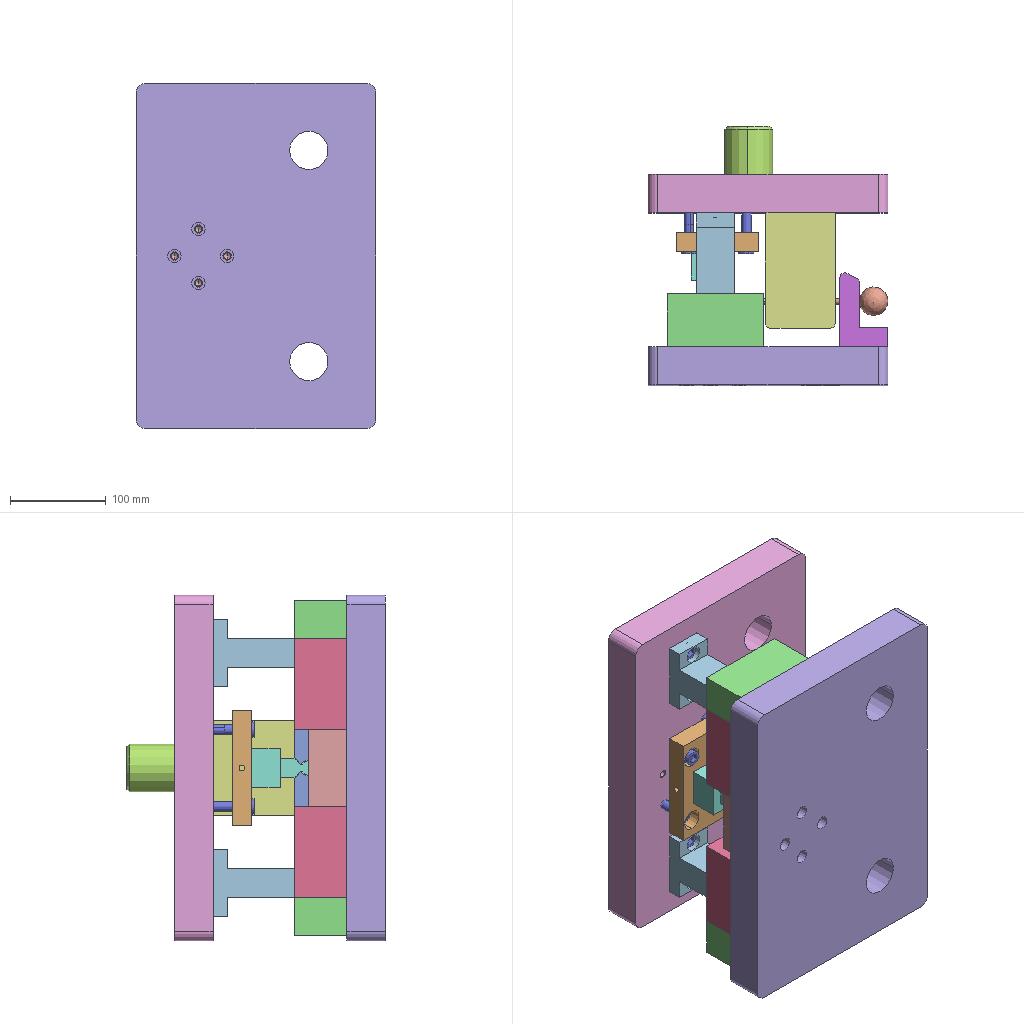Assembly | SolidWorks | 15 different items | 46 placed | box 250 x 270 x 360 mm
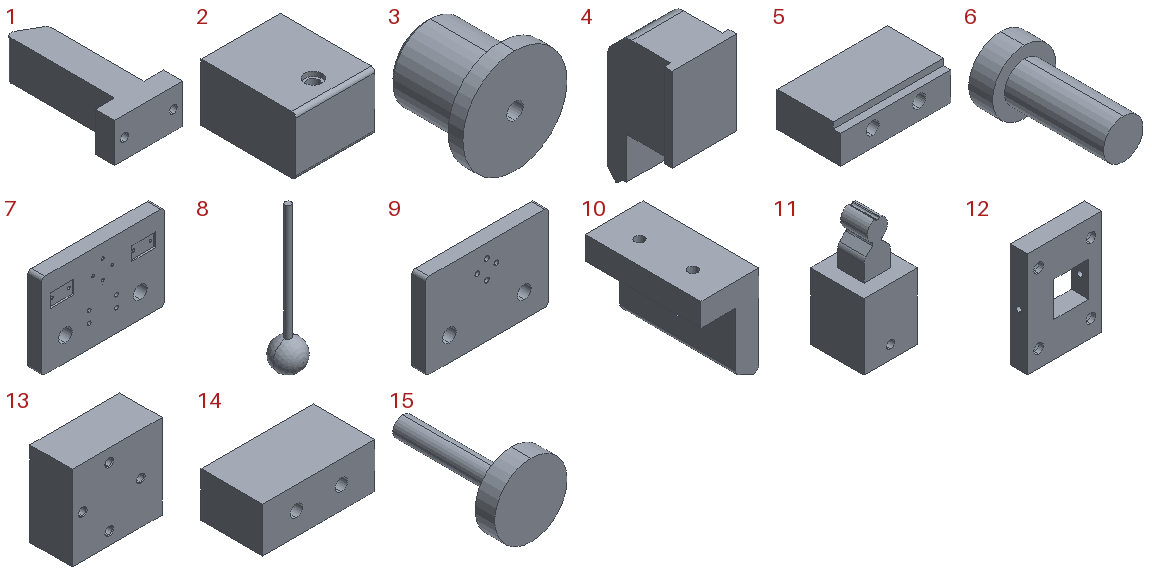Parts list (item | quantity | size | volume | features):
1 | x2 | 70 x 131.42 x 40 mm | 176977 mm3 | features ICE 3, Extrusion 1, Fillet 1, MoveFace 1
2 | x1 | 100 x 120 x 73 mm | 861044 mm3 | features ICE 3, MoveFace 2, Extrusion 1, Fillet 1, HoleWzd 1
3 | x1 | 70 x 60 x 70 mm | 128525 mm3 | features ICE 3, Chamfer 1, Extrusion 1
4 | x2 | 50 x 55 x 101.25 mm | 146000 mm3 | features ICE 3, Extrusion 1, Fillet 1
5 | x4 | 95 x 55 x 30 mm | 136523 mm3 | features ICE 3, Extrusion 1
6 | x26 | 16 x 31 x 16 mm | 2781 mm3 | features ICE 2, Extrusion 1
7 | x1 | 360 x 40 x 250 mm | 3399015 mm3 | features ICE 4, HoleWzd 3, Extrusion 1, MoveFace 1
8 | x1 | 30 x 30 x 145 mm | 17393 mm3 | features ICE 1, Revolution 1
9 | x1 | 360 x 40 x 250 mm | 3459963 mm3 | features Extrusion 1, HoleWzd 1, ICE 1
10 | x1 | 50 x 100 x 76.91 mm | 202541 mm3 | features ICE 4, Extrusion 1, Fillet 1
11 | x1 | 40 x 40 x 87.456 mm | 90363 mm3 | features ICE 3, Extrusion 1
12 | x1 | 85 x 20 x 120 mm | 147044 mm3 | features ICE 2, Extrusion 1
13 | x1 | 85 x 40 x 80 mm | 265399 mm3 | features ICE 2, Extrusion 1, HoleWzd 1
14 | x2 | 100 x 55 x 40 mm | 203169 mm3 | features Extrusion 1, ICE 1
15 | x1 | 22 x 39 x 22 mm | 3214 mm3 | features Extrusion 1, ICE 1
Mates (type | each side: item.copy, entity, surface, feature):
Concentric | 3.1 face cylinder Boss-Extrude1 | 7.1 face cylinder Cut-Extrude1
Coincident | 3.1 face plane Boss-Extrude1 | 7.1 face plane Cut-Extrude1
Coincident | 13.1 face plane Boss-Extrude1 | 9.1 face plane Boss-Extrude1
Concentric | 13.1 face cylinder M8 Tapped Hole1 | 9.1 face cylinder Boss-Extrude1 | 2 times
Parallel | 13.1 face cylinder M8 Tapped Hole1 | 9.1 face cylinder Boss-Extrude1
Coincident | 4.1 face plane Boss-Extrude1 | 9.1 face plane Boss-Extrude1
Coincident | 13.1 face plane Boss-Extrude1 | 4.1 face plane Boss-Extrude1
Coincident | 9.1 face plane Boss-Extrude1 | 4.2 face plane Boss-Extrude1
Coincident | 13.1 face plane Boss-Extrude1 | 4.2 face plane Boss-Extrude1
Coincident | 11.1 face plane Boss-Extrude1 | 12.1 face plane Boss-Extrude1 | 2 times
Coincident | 11.1 face plane Boss-Extrude3 | 12.1 face plane Boss-Extrude1
Parallel | 7.1 face plane Boss-Extrude1 | 9.1 face plane Boss-Extrude1
Coincident | 7.1 face plane Boss-Extrude1 | 9.1 face plane Boss-Extrude1
Concentric | 13.1 face cylinder Cut-Extrude2 | 11.1 face cylinder Boss-Extrude1
Coincident | 9.1 face plane Boss-Extrude1 | 14.1 face plane Boss-Extrude1
Concentric | 9.1 face cylinder M10 Tapped Hole1 | 14.1 face cylinder Cut-Extrude1 | 2 times
Coincident | 9.1 face plane Boss-Extrude1 | 14.2 face plane Boss-Extrude1
Concentric | 9.1 face cylinder M10 Tapped Hole1 | 14.2 edge
Concentric | 9.1 face cylinder M10 Tapped Hole1 | 14.2 face cylinder Cut-Extrude1
Coincident | 9.1 face plane Boss-Extrude1 | 5.1 face plane Boss-Extrude1
Concentric | 9.1 face cylinder M10 Tapped Hole1 | 5.1 face cylinder Cut-Extrude2 | 2 times
Coincident | 9.1 face plane Boss-Extrude1 | 5.2 face plane Boss-Extrude1
Concentric | 9.1 face cylinder M10 Tapped Hole1 | 5.2 face cylinder Cut-Extrude2 | 2 times
Coincident | 9.1 face plane Boss-Extrude1 | 5.3 face plane Boss-Extrude1
Concentric | 9.1 face cylinder M10 Tapped Hole1 | 5.3 face cylinder Cut-Extrude2 | 2 times
Coincident | 9.1 face plane Boss-Extrude1 | 5.4 face plane Boss-Extrude1
Concentric | 9.1 face cylinder M10 Tapped Hole1 | 5.4 face cylinder Cut-Extrude2 | 2 times
Coincident | 7.1 face plane Cut-Extrude3 | 1.1 face plane Boss-Extrude1
Concentric | 7.1 face cylinder M8 Tapped Hole4 | 1.1 face cylinder Boss-Extrude1 | 2 times
Coincident | 7.1 face plane Cut-Extrude3 | 1.2 face plane Boss-Extrude1
Concentric | 7.1 face cylinder M8 Tapped Hole4 | 1.2 face cylinder Boss-Extrude1 | 2 times
Coincident | 7.1 face plane Boss-Extrude1 | 2.1 face plane Boss-Extrude1
Concentric | 7.1 edge | 2.1 face cylinder M10 Tapped Hole1
Concentric | 7.1 face cylinder Cut-Extrude2 | 2.1 face cylinder M10 Tapped Hole1
Coincident | 9.1 face plane Boss-Extrude1 | 10.1 face plane Boss-Extrude1
Concentric | 9.1 face cylinder M10 Tapped Hole1 | 10.1 face cylinder Cut-Extrude3 | 2 times
Coincident | 2.1 face plane Cut-Extrude2 | 15.1 face plane Boss-Extrude1
Concentric | 2.1 face cylinder Cut-Extrude3 | 15.1 face cylinder Boss-Extrude2
Concentric | 10.1 face cylinder Cut-Extrude1 | 8.1 face cylinder Boss-Extrude1
Tangent | 10.1 face plane Boss-Extrude1 | 8.1 face sphere Revolve3
Concentric | 14.2 face cylinder Cut-Extrude1 | 6.1 face cylinder Boss-Extrude1
Concentric | 14.2 face cylinder Cut-Extrude1 | 6.2 face cylinder Boss-Extrude1
Concentric | 5.4 face cylinder Cut-Extrude2 | 6.3 face cylinder Boss-Extrude1
Concentric | 5.4 face cylinder Cut-Extrude2 | 6.4 face cylinder Boss-Extrude1
Concentric | 5.3 face cylinder Cut-Extrude2 | 6.5 face cylinder Boss-Extrude1
Concentric | 5.3 face cylinder Cut-Extrude2 | 6.6 face cylinder Boss-Extrude1
Concentric | 5.2 face cylinder Cut-Extrude2 | 6.7 face cylinder Boss-Extrude1
Concentric | 5.2 face cylinder Cut-Extrude2 | 6.8 face cylinder Boss-Extrude1
Concentric | 14.1 face cylinder Cut-Extrude1 | 6.9 face cylinder Boss-Extrude1
Concentric | 14.1 face cylinder Cut-Extrude1 | 6.10 face cylinder Boss-Extrude1
Concentric | 5.1 edge | 6.11 face cylinder Boss-Extrude1
Concentric | 5.1 face cylinder Cut-Extrude2 | 6.12 face cylinder Boss-Extrude1
Concentric | 10.1 face cylinder Cut-Extrude3 | 6.13 face cylinder Boss-Extrude1
Coincident | 5.2 face plane Cut-Extrude2 | 6.7 face plane Cut-Extrude1
Coincident | 5.2 face plane Cut-Extrude2 | 6.8 face plane Cut-Extrude1
Coincident | 14.1 face plane Cut-Extrude1 | 6.9 face plane Cut-Extrude1
Coincident | 14.1 face plane Cut-Extrude1 | 6.10 face plane Cut-Extrude1
Coincident | 14.2 face plane Cut-Extrude1 | 6.2 face plane Cut-Extrude1
Coincident | 14.2 face plane Cut-Extrude1 | 6.1 face plane Cut-Extrude1
Coincident | 5.3 face plane Cut-Extrude2 | 6.5 face plane Cut-Extrude1
Coincident | 5.3 face plane Cut-Extrude2 | 6.6 face plane Cut-Extrude1
Coincident | 5.1 face plane Cut-Extrude2 | 6.12 face plane Cut-Extrude1
Coincident | 5.1 face plane Cut-Extrude2 | 6.11 face plane Cut-Extrude1
Coincident | 10.1 face plane Cut-Extrude3 | 6.13 face plane Cut-Extrude1
Coincident | 10.1 face plane Cut-Extrude3 | 6.14 face plane Cut-Extrude1
Concentric | 10.1 face cylinder Cut-Extrude3 | 6.14 face cylinder Boss-Extrude2
Concentric | 7.1 face cylinder Cut-Extrude2 | 6.15 face cylinder Boss-Extrude1
Concentric | 7.1 face cylinder Cut-Extrude2 | 6.16 face cylinder Boss-Extrude1
Concentric | 7.1 face cylinder Cut-Extrude2 | 6.17 face cylinder Boss-Extrude1
Concentric | 7.1 face cylinder Cut-Extrude2 | 6.18 face cylinder Boss-Extrude1
Coincident | 7.1 face plane Cut-Extrude2 | 6.18 face plane Cut-Extrude1
Coincident | 7.1 face plane Cut-Extrude2 | 6.17 face plane Cut-Extrude1
Coincident | 7.1 face plane Cut-Extrude2 | 6.16 face plane Cut-Extrude1
Coincident | 7.1 face plane Cut-Extrude2 | 6.15 face plane Cut-Extrude1
Concentric | 1.2 face cylinder Cut-Extrude2 | 6.19 face cylinder Boss-Extrude1
Concentric | 1.2 face cylinder Cut-Extrude2 | 6.20 face cylinder Boss-Extrude1
Concentric | 12.1 edge | 6.21 face cylinder Boss-Extrude1
Concentric | 12.1 face cylinder Cut-Extrude1 | 6.22 face cylinder Boss-Extrude1
Concentric | 12.1 face cylinder Cut-Extrude1 | 6.23 face cylinder Boss-Extrude1
Concentric | 12.1 face cylinder Cut-Extrude1 | 6.24 face cylinder Boss-Extrude1
Coincident | 1.2 face plane Cut-Extrude2 | 6.19 face plane Cut-Extrude1
Coincident | 1.2 face plane Cut-Extrude2 | 6.20 face plane Cut-Extrude1
Coincident | 12.1 face plane Cut-Extrude1 | 6.21 face plane Cut-Extrude1
Coincident | 12.1 face plane Cut-Extrude1 | 6.23 face plane Cut-Extrude1
Coincident | 6.24 face plane Cut-Extrude1 | 6.22 edge
Concentric | 1.1 face cylinder Cut-Extrude2 | 6.25 face cylinder Boss-Extrude2
Concentric | 1.1 face cylinder Cut-Extrude2 | 6.26 face cylinder Boss-Extrude2
Coincident | 1.1 face plane Cut-Extrude2 | 6.26 face plane Cut-Extrude1
Coincident | 1.1 face plane Cut-Extrude2 | 6.25 face plane Cut-Extrude1
Coincident | 5.4 face plane Cut-Extrude2 | 6.3 face plane Cut-Extrude1
Coincident | 5.4 face plane Cut-Extrude2 | 6.4 face plane Cut-Extrude1